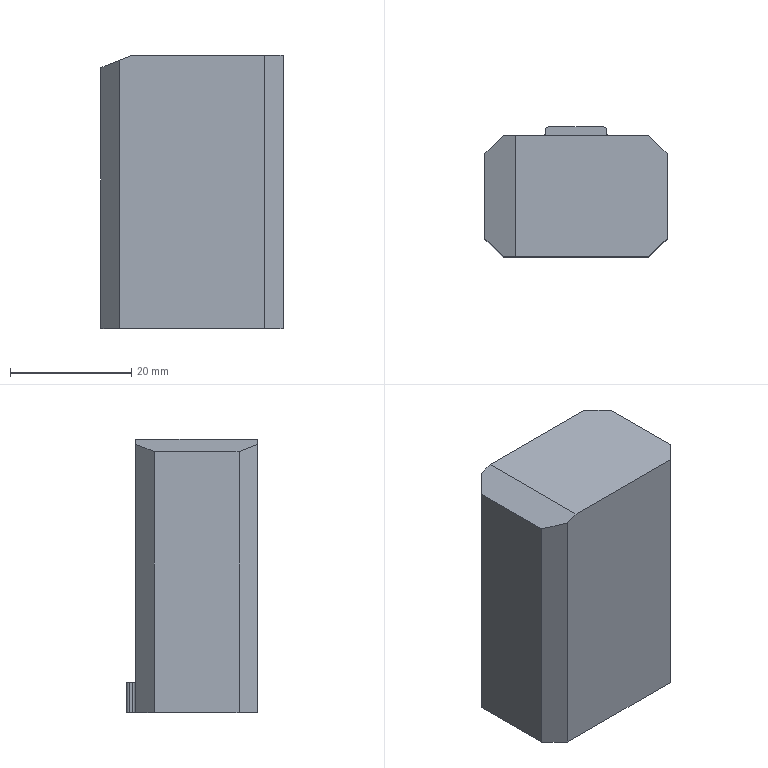Part | NX | features DIE-57 2 | 1 solid | 21 faces | box 30 x 21.5 x 45 mm | volume 25409 mm3 | plane 16 | cylinder 5 | commonest cylinder face diameters 1 x4 14.003 x1
STEP:
#1=CARTESIAN_POINT('',(3135.094,-901.123,858.716));
#2=VERTEX_POINT('',#1);
#3=CARTESIAN_POINT('',(3157.094,-901.123,858.716));
#4=VERTEX_POINT('',#3);
#5=CARTESIAN_POINT('',(3145.094,-901.123,858.716));
#6=DIRECTION('',(1.,0.,0.));
#7=VECTOR('',#6,1000.);
#8=LINE('',#5,#7);
#9=EDGE_CURVE('',#2,#4,#8,.T.);
#10=ORIENTED_EDGE('',*,*,#9,.T.);
#11=CARTESIAN_POINT('',(3160.094,-898.123,858.716));
#12=VERTEX_POINT('',#11);
#13=CARTESIAN_POINT('',(3153.594,-904.623,858.716));
#14=DIRECTION('',(0.7071,0.7071,0.));
#15=VECTOR('',#14,1000.);
#16=LINE('',#13,#15);
#17=EDGE_CURVE('',#12,#4,#16,.F.);
#18=ORIENTED_EDGE('',*,*,#17,.F.);
#19=CARTESIAN_POINT('',(3160.094,-884.123,858.716));
#20=VERTEX_POINT('',#19);
#21=CARTESIAN_POINT('',(3160.094,-891.123,858.716));
#22=DIRECTION('',(0.,1.,0.));
#23=VECTOR('',#22,1000.);
#24=LINE('',#21,#23);
#25=EDGE_CURVE('',#12,#20,#24,.T.);
#26=ORIENTED_EDGE('',*,*,#25,.T.);
#27=CARTESIAN_POINT('',(3157.094,-881.123,858.716));
#28=VERTEX_POINT('',#27);
#29=CARTESIAN_POINT('',(3153.594,-877.623,858.716));
#30=DIRECTION('',(-0.7071,0.7071,0.));
#31=VECTOR('',#30,1000.);
#32=LINE('',#29,#31);
#33=EDGE_CURVE('',#28,#20,#32,.F.);
#34=ORIENTED_EDGE('',*,*,#33,.F.);
#35=CARTESIAN_POINT('',(3135.094,-881.123,858.716));
#36=VERTEX_POINT('',#35);
#37=CARTESIAN_POINT('',(3145.094,-881.123,858.716));
#38=DIRECTION('',(-1.,0.,0.));
#39=VECTOR('',#38,1000.);
#40=LINE('',#37,#39);
#41=EDGE_CURVE('',#28,#36,#40,.T.);
#42=ORIENTED_EDGE('',*,*,#41,.T.);
#43=CARTESIAN_POINT('',(3135.094,-891.123,858.716));
#44=DIRECTION('',(0.,1.,0.));
#45=VECTOR('',#44,1000.);
#46=LINE('',#43,#45);
#47=EDGE_CURVE('',#2,#36,#46,.T.);
#48=ORIENTED_EDGE('',*,*,#47,.F.);
#49=EDGE_LOOP('',(#10,#18,#26,#34,#42,#48));
#50=FACE_BOUND('',#49,.T.);
#51=CARTESIAN_POINT('',(3145.094,-891.123,858.716));
#52=DIRECTION('',(0.,0.,1.));
#53=DIRECTION('',(1.,0.,0.));
#54=AXIS2_PLACEMENT_3D('',#51,#52,#53);
#55=PLANE('',#54);
#56=ADVANCED_FACE('',(#50),#55,.T.);
#57=CARTESIAN_POINT('',(3139.594,-881.123,818.716));
#58=VERTEX_POINT('',#57);
#59=CARTESIAN_POINT('',(3150.594,-881.123,818.716));
#60=VERTEX_POINT('',#59);
#61=CARTESIAN_POINT('',(3145.094,-881.123,818.716));
#62=DIRECTION('',(1.,0.,0.));
#63=VECTOR('',#62,1000.);
#64=LINE('',#61,#63);
#65=EDGE_CURVE('',#58,#60,#64,.T.);
#66=ORIENTED_EDGE('',*,*,#65,.F.);
#67=CARTESIAN_POINT('',(3139.594,-881.123,813.716));
#68=VERTEX_POINT('',#67);
#69=CARTESIAN_POINT('',(3139.594,-881.123,818.716));
#70=DIRECTION('',(0.,0.,-1.));
#71=VECTOR('',#70,1000.);
#72=LINE('',#69,#71);
#73=EDGE_CURVE('',#68,#58,#72,.F.);
#74=ORIENTED_EDGE('',*,*,#73,.F.);
#75=CARTESIAN_POINT('',(3133.094,-881.123,813.716));
#76=VERTEX_POINT('',#75);
#77=CARTESIAN_POINT('',(3145.094,-881.123,813.716));
#78=DIRECTION('',(1.,0.,0.));
#79=VECTOR('',#78,1000.);
#80=LINE('',#77,#79);
#81=EDGE_CURVE('',#76,#68,#80,.T.);
#82=ORIENTED_EDGE('',*,*,#81,.F.);
#83=CARTESIAN_POINT('',(3133.094,-881.123,857.916));
#84=VERTEX_POINT('',#83);
#85=CARTESIAN_POINT('',(3133.094,-881.123,823.716));
#86=DIRECTION('',(0.,0.,-1.));
#87=VECTOR('',#86,1000.);
#88=LINE('',#85,#87);
#89=EDGE_CURVE('',#84,#76,#88,.T.);
#90=ORIENTED_EDGE('',*,*,#89,.F.);
#91=CARTESIAN_POINT('',(3135.956,-881.123,859.061));
#92=DIRECTION('',(0.9285,0.,0.3714));
#93=VECTOR('',#92,1000.);
#94=LINE('',#91,#93);
#95=EDGE_CURVE('',#36,#84,#94,.F.);
#96=ORIENTED_EDGE('',*,*,#95,.F.);
#97=ORIENTED_EDGE('',*,*,#41,.F.);
#98=CARTESIAN_POINT('',(3157.094,-881.123,813.716));
#99=VERTEX_POINT('',#98);
#100=CARTESIAN_POINT('',(3157.094,-881.123,823.716));
#101=DIRECTION('',(0.,0.,1.));
#102=VECTOR('',#101,1000.);
#103=LINE('',#100,#102);
#104=EDGE_CURVE('',#99,#28,#103,.T.);
#105=ORIENTED_EDGE('',*,*,#104,.F.);
#106=CARTESIAN_POINT('',(3150.594,-881.123,813.716));
#107=VERTEX_POINT('',#106);
#108=CARTESIAN_POINT('',(3145.094,-881.123,813.716));
#109=DIRECTION('',(1.,0.,0.));
#110=VECTOR('',#109,1000.);
#111=LINE('',#108,#110);
#112=EDGE_CURVE('',#107,#99,#111,.T.);
#113=ORIENTED_EDGE('',*,*,#112,.F.);
#114=CARTESIAN_POINT('',(3150.594,-881.123,813.716));
#115=DIRECTION('',(0.,0.,1.));
#116=VECTOR('',#115,1000.);
#117=LINE('',#114,#116);
#118=EDGE_CURVE('',#60,#107,#117,.F.);
#119=ORIENTED_EDGE('',*,*,#118,.F.);
#120=EDGE_LOOP('',(#66,#74,#82,#90,#96,#97,#105,#113,#119));
#121=FACE_BOUND('',#120,.T.);
#122=CARTESIAN_POINT('',(3145.094,-881.123,823.716));
#123=DIRECTION('',(0.,1.,0.));
#124=DIRECTION('',(0.,0.,-1.));
#125=AXIS2_PLACEMENT_3D('',#122,#123,#124);
#126=PLANE('',#125);
#127=ADVANCED_FACE('',(#121),#126,.T.);
#128=CARTESIAN_POINT('',(3130.094,-884.123,813.716));
#129=VERTEX_POINT('',#128);
#130=CARTESIAN_POINT('',(3130.094,-884.123,856.716));
#131=VERTEX_POINT('',#130);
#132=CARTESIAN_POINT('',(3130.094,-884.123,823.716));
#133=DIRECTION('',(0.,0.,1.));
#134=VECTOR('',#133,1000.);
#135=LINE('',#132,#134);
#136=EDGE_CURVE('',#129,#131,#135,.T.);
#137=ORIENTED_EDGE('',*,*,#136,.F.);
#138=CARTESIAN_POINT('',(3130.094,-898.123,813.716));
#139=VERTEX_POINT('',#138);
#140=CARTESIAN_POINT('',(3130.094,-891.123,813.716));
#141=DIRECTION('',(0.,1.,0.));
#142=VECTOR('',#141,1000.);
#143=LINE('',#140,#142);
#144=EDGE_CURVE('',#139,#129,#143,.T.);
#145=ORIENTED_EDGE('',*,*,#144,.F.);
#146=CARTESIAN_POINT('',(3130.094,-898.123,856.716));
#147=VERTEX_POINT('',#146);
#148=CARTESIAN_POINT('',(3130.094,-898.123,823.716));
#149=DIRECTION('',(0.,0.,-1.));
#150=VECTOR('',#149,1000.);
#151=LINE('',#148,#150);
#152=EDGE_CURVE('',#147,#139,#151,.T.);
#153=ORIENTED_EDGE('',*,*,#152,.F.);
#154=CARTESIAN_POINT('',(3130.094,-891.123,856.716));
#155=DIRECTION('',(0.,-1.,0.));
#156=VECTOR('',#155,1000.);
#157=LINE('',#154,#156);
#158=EDGE_CURVE('',#131,#147,#157,.T.);
#159=ORIENTED_EDGE('',*,*,#158,.F.);
#160=EDGE_LOOP('',(#137,#145,#153,#159));
#161=FACE_BOUND('',#160,.T.);
#162=CARTESIAN_POINT('',(3130.094,-891.123,823.716));
#163=DIRECTION('',(-1.,0.,0.));
#164=DIRECTION('',(0.,0.,1.));
#165=AXIS2_PLACEMENT_3D('',#162,#163,#164);
#166=PLANE('',#165);
#167=ADVANCED_FACE('',(#161),#166,.T.);
#168=CARTESIAN_POINT('',(3133.094,-901.123,813.716));
#169=VERTEX_POINT('',#168);
#170=CARTESIAN_POINT('',(3133.094,-901.123,857.916));
#171=VERTEX_POINT('',#170);
#172=CARTESIAN_POINT('',(3133.094,-901.123,823.716));
#173=DIRECTION('',(0.,0.,1.));
#174=VECTOR('',#173,1000.);
#175=LINE('',#172,#174);
#176=EDGE_CURVE('',#169,#171,#175,.T.);
#177=ORIENTED_EDGE('',*,*,#176,.F.);
#178=CARTESIAN_POINT('',(3157.094,-901.123,813.716));
#179=VERTEX_POINT('',#178);
#180=CARTESIAN_POINT('',(3145.094,-901.123,813.716));
#181=DIRECTION('',(-1.,0.,0.));
#182=VECTOR('',#181,1000.);
#183=LINE('',#180,#182);
#184=EDGE_CURVE('',#179,#169,#183,.T.);
#185=ORIENTED_EDGE('',*,*,#184,.F.);
#186=CARTESIAN_POINT('',(3157.094,-901.123,823.716));
#187=DIRECTION('',(0.,0.,-1.));
#188=VECTOR('',#187,1000.);
#189=LINE('',#186,#188);
#190=EDGE_CURVE('',#4,#179,#189,.T.);
#191=ORIENTED_EDGE('',*,*,#190,.F.);
#192=ORIENTED_EDGE('',*,*,#9,.F.);
#193=CARTESIAN_POINT('',(3135.956,-901.123,859.061));
#194=DIRECTION('',(-0.9285,0.,-0.3714));
#195=VECTOR('',#194,1000.);
#196=LINE('',#193,#195);
#197=EDGE_CURVE('',#171,#2,#196,.F.);
#198=ORIENTED_EDGE('',*,*,#197,.F.);
#199=EDGE_LOOP('',(#177,#185,#191,#192,#198));
#200=FACE_BOUND('',#199,.T.);
#201=CARTESIAN_POINT('',(3145.094,-901.123,823.716));
#202=DIRECTION('',(0.,-1.,0.));
#203=DIRECTION('',(0.,0.,1.));
#204=AXIS2_PLACEMENT_3D('',#201,#202,#203);
#205=PLANE('',#204);
#206=ADVANCED_FACE('',(#200),#205,.T.);
#207=CARTESIAN_POINT('',(3138.092,-891.123,813.716));
#208=VERTEX_POINT('',#207);
#209=CARTESIAN_POINT('',(3145.094,-891.123,813.716));
#210=DIRECTION('',(0.,0.,-1.));
#211=DIRECTION('',(-1.,0.,0.));
#212=AXIS2_PLACEMENT_3D('',#209,#210,#211);
#213=CIRCLE('',#212,7.002);
#214=EDGE_CURVE('',#208,#208,#213,.F.);
#215=ORIENTED_EDGE('',*,*,#214,.T.);
#216=EDGE_LOOP('',(#215));
#217=FACE_BOUND('',#216,.T.);
#218=CARTESIAN_POINT('',(3150.094,-880.623,813.716));
#219=VERTEX_POINT('',#218);
#220=CARTESIAN_POINT('',(3150.094,-880.123,813.716));
#221=VERTEX_POINT('',#220);
#222=CARTESIAN_POINT('',(3150.094,-2118.745,813.716));
#223=DIRECTION('',(0.,1.,0.));
#224=VECTOR('',#223,1000.);
#225=LINE('',#222,#224);
#226=EDGE_CURVE('',#219,#221,#225,.T.);
#227=ORIENTED_EDGE('',*,*,#226,.F.);
#228=CARTESIAN_POINT('',(3150.594,-880.623,813.716));
#229=DIRECTION('',(0.,0.,1.));
#230=DIRECTION('',(-1.,0.,0.));
#231=AXIS2_PLACEMENT_3D('',#228,#229,#230);
#232=CIRCLE('',#231,0.5);
#233=EDGE_CURVE('',#107,#219,#232,.F.);
#234=ORIENTED_EDGE('',*,*,#233,.F.);
#235=ORIENTED_EDGE('',*,*,#112,.T.);
#236=CARTESIAN_POINT('',(3160.094,-884.123,813.716));
#237=VERTEX_POINT('',#236);
#238=CARTESIAN_POINT('',(3153.594,-877.623,813.716));
#239=DIRECTION('',(0.7071,-0.7071,0.));
#240=VECTOR('',#239,1000.);
#241=LINE('',#238,#240);
#242=EDGE_CURVE('',#237,#99,#241,.F.);
#243=ORIENTED_EDGE('',*,*,#242,.F.);
#244=CARTESIAN_POINT('',(3160.094,-898.123,813.716));
#245=VERTEX_POINT('',#244);
#246=CARTESIAN_POINT('',(3160.094,-891.123,813.716));
#247=DIRECTION('',(0.,-1.,0.));
#248=VECTOR('',#247,1000.);
#249=LINE('',#246,#248);
#250=EDGE_CURVE('',#237,#245,#249,.T.);
#251=ORIENTED_EDGE('',*,*,#250,.T.);
#252=CARTESIAN_POINT('',(3153.594,-904.623,813.716));
#253=DIRECTION('',(-0.7071,-0.7071,0.));
#254=VECTOR('',#253,1000.);
#255=LINE('',#252,#254);
#256=EDGE_CURVE('',#179,#245,#255,.F.);
#257=ORIENTED_EDGE('',*,*,#256,.F.);
#258=ORIENTED_EDGE('',*,*,#184,.T.);
#259=CARTESIAN_POINT('',(3136.594,-904.623,813.716));
#260=DIRECTION('',(-0.7071,0.7071,0.));
#261=VECTOR('',#260,1000.);
#262=LINE('',#259,#261);
#263=EDGE_CURVE('',#139,#169,#262,.F.);
#264=ORIENTED_EDGE('',*,*,#263,.F.);
#265=ORIENTED_EDGE('',*,*,#144,.T.);
#266=CARTESIAN_POINT('',(3136.594,-877.623,813.716));
#267=DIRECTION('',(0.7071,0.7071,0.));
#268=VECTOR('',#267,1000.);
#269=LINE('',#266,#268);
#270=EDGE_CURVE('',#76,#129,#269,.F.);
#271=ORIENTED_EDGE('',*,*,#270,.F.);
#272=ORIENTED_EDGE('',*,*,#81,.T.);
#273=CARTESIAN_POINT('',(3140.094,-880.623,813.716));
#274=VERTEX_POINT('',#273);
#275=CARTESIAN_POINT('',(3139.594,-880.623,813.716));
#276=DIRECTION('',(0.,0.,1.));
#277=DIRECTION('',(-1.,0.,0.));
#278=AXIS2_PLACEMENT_3D('',#275,#276,#277);
#279=CIRCLE('',#278,0.5);
#280=EDGE_CURVE('',#274,#68,#279,.F.);
#281=ORIENTED_EDGE('',*,*,#280,.F.);
#282=CARTESIAN_POINT('',(3140.094,-880.123,813.716));
#283=VERTEX_POINT('',#282);
#284=CARTESIAN_POINT('',(3140.094,-2118.745,813.716));
#285=DIRECTION('',(0.,-1.,0.));
#286=VECTOR('',#285,1000.);
#287=LINE('',#284,#286);
#288=EDGE_CURVE('',#283,#274,#287,.T.);
#289=ORIENTED_EDGE('',*,*,#288,.F.);
#290=CARTESIAN_POINT('',(3140.594,-879.623,813.716));
#291=VERTEX_POINT('',#290);
#292=CARTESIAN_POINT('',(3140.594,-880.123,813.716));
#293=DIRECTION('',(0.,0.,1.));
#294=DIRECTION('',(-1.,0.,0.));
#295=AXIS2_PLACEMENT_3D('',#292,#293,#294);
#296=CIRCLE('',#295,0.5);
#297=EDGE_CURVE('',#291,#283,#296,.T.);
#298=ORIENTED_EDGE('',*,*,#297,.F.);
#299=CARTESIAN_POINT('',(3149.594,-879.623,813.716));
#300=VERTEX_POINT('',#299);
#301=CARTESIAN_POINT('',(3145.094,-879.623,813.716));
#302=DIRECTION('',(-1.,0.,0.));
#303=VECTOR('',#302,1000.);
#304=LINE('',#301,#303);
#305=EDGE_CURVE('',#300,#291,#304,.T.);
#306=ORIENTED_EDGE('',*,*,#305,.F.);
#307=CARTESIAN_POINT('',(3149.594,-880.123,813.716));
#308=DIRECTION('',(0.,0.,1.));
#309=DIRECTION('',(-1.,0.,0.));
#310=AXIS2_PLACEMENT_3D('',#307,#308,#309);
#311=CIRCLE('',#310,0.5);
#312=EDGE_CURVE('',#221,#300,#311,.T.);
#313=ORIENTED_EDGE('',*,*,#312,.F.);
#314=EDGE_LOOP('',(#227,#234,#235,#243,#251,#257,#258,#264,#265,#271,#272,#281,#289,#298,#306,#313));
#315=FACE_BOUND('',#314,.T.);
#316=CARTESIAN_POINT('',(3145.094,-891.123,813.716));
#317=DIRECTION('',(0.,0.,-1.));
#318=DIRECTION('',(-1.,0.,0.));
#319=AXIS2_PLACEMENT_3D('',#316,#317,#318);
#320=PLANE('',#319);
#321=ADVANCED_FACE('',(#217,#315),#320,.T.);
#322=ORIENTED_EDGE('',*,*,#25,.F.);
#323=CARTESIAN_POINT('',(3160.094,-898.123,823.716));
#324=DIRECTION('',(0.,0.,1.));
#325=VECTOR('',#324,1000.);
#326=LINE('',#323,#325);
#327=EDGE_CURVE('',#245,#12,#326,.T.);
#328=ORIENTED_EDGE('',*,*,#327,.F.);
#329=ORIENTED_EDGE('',*,*,#250,.F.);
#330=CARTESIAN_POINT('',(3160.094,-884.123,823.716));
#331=DIRECTION('',(0.,0.,-1.));
#332=VECTOR('',#331,1000.);
#333=LINE('',#330,#332);
#334=EDGE_CURVE('',#20,#237,#333,.T.);
#335=ORIENTED_EDGE('',*,*,#334,.F.);
#336=EDGE_LOOP('',(#322,#328,#329,#335));
#337=FACE_BOUND('',#336,.T.);
#338=CARTESIAN_POINT('',(3160.094,-891.123,823.716));
#339=DIRECTION('',(1.,0.,0.));
#340=DIRECTION('',(0.,0.,-1.));
#341=AXIS2_PLACEMENT_3D('',#338,#339,#340);
#342=PLANE('',#341);
#343=ADVANCED_FACE('',(#337),#342,.T.);
#344=ORIENTED_EDGE('',*,*,#242,.T.);
#345=ORIENTED_EDGE('',*,*,#104,.T.);
#346=ORIENTED_EDGE('',*,*,#33,.T.);
#347=ORIENTED_EDGE('',*,*,#334,.T.);
#348=EDGE_LOOP('',(#344,#345,#346,#347));
#349=FACE_BOUND('',#348,.T.);
#350=CARTESIAN_POINT('',(3157.094,-881.123,823.716));
#351=DIRECTION('',(-0.7071,-0.7071,0.));
#352=DIRECTION('',(0.,0.,1.));
#353=AXIS2_PLACEMENT_3D('',#350,#351,#352);
#354=PLANE('',#353);
#355=ADVANCED_FACE('',(#349),#354,.F.);
#356=ORIENTED_EDGE('',*,*,#256,.T.);
#357=ORIENTED_EDGE('',*,*,#327,.T.);
#358=ORIENTED_EDGE('',*,*,#17,.T.);
#359=ORIENTED_EDGE('',*,*,#190,.T.);
#360=EDGE_LOOP('',(#356,#357,#358,#359));
#361=FACE_BOUND('',#360,.T.);
#362=CARTESIAN_POINT('',(3160.094,-898.123,823.716));
#363=DIRECTION('',(-0.7071,0.7071,0.));
#364=DIRECTION('',(0.,0.,1.));
#365=AXIS2_PLACEMENT_3D('',#362,#363,#364);
#366=PLANE('',#365);
#367=ADVANCED_FACE('',(#361),#366,.F.);
#368=ORIENTED_EDGE('',*,*,#152,.T.);
#369=ORIENTED_EDGE('',*,*,#263,.T.);
#370=ORIENTED_EDGE('',*,*,#176,.T.);
#371=CARTESIAN_POINT('',(3126.761,-894.789,855.383));
#372=DIRECTION('',(0.6804,-0.6804,0.2722));
#373=VECTOR('',#372,1000.);
#374=LINE('',#371,#373);
#375=EDGE_CURVE('',#147,#171,#374,.T.);
#376=ORIENTED_EDGE('',*,*,#375,.F.);
#377=EDGE_LOOP('',(#368,#369,#370,#376));
#378=FACE_BOUND('',#377,.T.);
#379=CARTESIAN_POINT('',(3133.094,-901.123,823.716));
#380=DIRECTION('',(0.7071,0.7071,0.));
#381=DIRECTION('',(0.,0.,1.));
#382=AXIS2_PLACEMENT_3D('',#379,#380,#381);
#383=PLANE('',#382);
#384=ADVANCED_FACE('',(#378),#383,.F.);
#385=ORIENTED_EDGE('',*,*,#89,.T.);
#386=ORIENTED_EDGE('',*,*,#270,.T.);
#387=ORIENTED_EDGE('',*,*,#136,.T.);
#388=CARTESIAN_POINT('',(3123.983,-890.234,854.272));
#389=DIRECTION('',(-0.6804,-0.6804,-0.2722));
#390=VECTOR('',#389,1000.);
#391=LINE('',#388,#390);
#392=EDGE_CURVE('',#84,#131,#391,.T.);
#393=ORIENTED_EDGE('',*,*,#392,.F.);
#394=EDGE_LOOP('',(#385,#386,#387,#393));
#395=FACE_BOUND('',#394,.T.);
#396=CARTESIAN_POINT('',(3130.094,-884.123,823.716));
#397=DIRECTION('',(0.7071,-0.7071,0.));
#398=DIRECTION('',(0.,0.,1.));
#399=AXIS2_PLACEMENT_3D('',#396,#397,#398);
#400=PLANE('',#399);
#401=ADVANCED_FACE('',(#395),#400,.F.);
#402=ORIENTED_EDGE('',*,*,#95,.T.);
#403=ORIENTED_EDGE('',*,*,#392,.T.);
#404=ORIENTED_EDGE('',*,*,#158,.T.);
#405=ORIENTED_EDGE('',*,*,#375,.T.);
#406=ORIENTED_EDGE('',*,*,#197,.T.);
#407=ORIENTED_EDGE('',*,*,#47,.T.);
#408=EDGE_LOOP('',(#402,#403,#404,#405,#406,#407));
#409=FACE_BOUND('',#408,.T.);
#410=CARTESIAN_POINT('',(3130.094,-891.123,856.716));
#411=DIRECTION('',(0.3714,0.,-0.9285));
#412=DIRECTION('',(0.,-1.,0.));
#413=AXIS2_PLACEMENT_3D('',#410,#411,#412);
#414=PLANE('',#413);
#415=ADVANCED_FACE('',(#409),#414,.F.);
#416=CARTESIAN_POINT('',(3140.094,-880.123,818.716));
#417=VERTEX_POINT('',#416);
#418=CARTESIAN_POINT('',(3140.094,-880.623,818.716));
#419=VERTEX_POINT('',#418);
#420=CARTESIAN_POINT('',(3140.094,-2118.745,818.716));
#421=DIRECTION('',(0.,-1.,0.));
#422=VECTOR('',#421,1000.);
#423=LINE('',#420,#422);
#424=EDGE_CURVE('',#417,#419,#423,.T.);
#425=ORIENTED_EDGE('',*,*,#424,.F.);
#426=CARTESIAN_POINT('',(3140.094,-880.123,818.716));
#427=DIRECTION('',(0.,0.,-1.));
#428=VECTOR('',#427,1000.);
#429=LINE('',#426,#428);
#430=EDGE_CURVE('',#283,#417,#429,.F.);
#431=ORIENTED_EDGE('',*,*,#430,.F.);
#432=ORIENTED_EDGE('',*,*,#288,.T.);
#433=CARTESIAN_POINT('',(3140.094,-880.623,813.716));
#434=DIRECTION('',(0.,0.,-1.));
#435=VECTOR('',#434,1000.);
#436=LINE('',#433,#435);
#437=EDGE_CURVE('',#419,#274,#436,.T.);
#438=ORIENTED_EDGE('',*,*,#437,.F.);
#439=EDGE_LOOP('',(#425,#431,#432,#438));
#440=FACE_BOUND('',#439,.T.);
#441=CARTESIAN_POINT('',(3140.094,-880.123,818.716));
#442=DIRECTION('',(-1.,0.,0.));
#443=DIRECTION('',(0.,0.,1.));
#444=AXIS2_PLACEMENT_3D('',#441,#442,#443);
#445=PLANE('',#444);
#446=ADVANCED_FACE('',(#440),#445,.T.);
#447=CARTESIAN_POINT('',(3150.094,-880.623,818.716));
#448=VERTEX_POINT('',#447);
#449=CARTESIAN_POINT('',(3150.094,-880.123,818.716));
#450=VERTEX_POINT('',#449);
#451=CARTESIAN_POINT('',(3150.094,-2118.745,818.716));
#452=DIRECTION('',(0.,1.,0.));
#453=VECTOR('',#452,1000.);
#454=LINE('',#451,#453);
#455=EDGE_CURVE('',#448,#450,#454,.T.);
#456=ORIENTED_EDGE('',*,*,#455,.F.);
#457=CARTESIAN_POINT('',(3150.094,-880.623,818.716));
#458=DIRECTION('',(0.,0.,1.));
#459=VECTOR('',#458,1000.);
#460=LINE('',#457,#459);
#461=EDGE_CURVE('',#219,#448,#460,.T.);
#462=ORIENTED_EDGE('',*,*,#461,.F.);
#463=ORIENTED_EDGE('',*,*,#226,.T.);
#464=CARTESIAN_POINT('',(3150.094,-880.123,818.716));
#465=DIRECTION('',(0.,0.,-1.));
#466=VECTOR('',#465,1000.);
#467=LINE('',#464,#466);
#468=EDGE_CURVE('',#450,#221,#467,.T.);
#469=ORIENTED_EDGE('',*,*,#468,.F.);
#470=EDGE_LOOP('',(#456,#462,#463,#469));
#471=FACE_BOUND('',#470,.T.);
#472=CARTESIAN_POINT('',(3150.094,-881.173,818.716));
#473=DIRECTION('',(1.,0.,0.));
#474=DIRECTION('',(0.,0.,-1.));
#475=AXIS2_PLACEMENT_3D('',#472,#473,#474);
#476=PLANE('',#475);
#477=ADVANCED_FACE('',(#471),#476,.T.);
#478=ORIENTED_EDGE('',*,*,#305,.T.);
#479=CARTESIAN_POINT('',(3140.594,-879.623,818.716));
#480=VERTEX_POINT('',#479);
#481=CARTESIAN_POINT('',(3140.594,-879.623,818.716));
#482=DIRECTION('',(0.,0.,-1.));
#483=VECTOR('',#482,1000.);
#484=LINE('',#481,#483);
#485=EDGE_CURVE('',#480,#291,#484,.T.);
#486=ORIENTED_EDGE('',*,*,#485,.F.);
#487=CARTESIAN_POINT('',(3149.594,-879.623,818.716));
#488=VERTEX_POINT('',#487);
#489=CARTESIAN_POINT('',(962.5,-879.623,818.716));
#490=DIRECTION('',(-1.,0.,0.));
#491=VECTOR('',#490,1000.);
#492=LINE('',#489,#491);
#493=EDGE_CURVE('',#488,#480,#492,.T.);
#494=ORIENTED_EDGE('',*,*,#493,.F.);
#495=CARTESIAN_POINT('',(3149.594,-879.623,818.716));
#496=DIRECTION('',(0.,0.,-1.));
#497=VECTOR('',#496,1000.);
#498=LINE('',#495,#497);
#499=EDGE_CURVE('',#300,#488,#498,.F.);
#500=ORIENTED_EDGE('',*,*,#499,.F.);
#501=EDGE_LOOP('',(#478,#486,#494,#500));
#502=FACE_BOUND('',#501,.T.);
#503=CARTESIAN_POINT('',(3162.094,-879.623,818.716));
#504=DIRECTION('',(0.,1.,0.));
#505=DIRECTION('',(0.,0.,-1.));
#506=AXIS2_PLACEMENT_3D('',#503,#504,#505);
#507=PLANE('',#506);
#508=ADVANCED_FACE('',(#502),#507,.T.);
#509=ORIENTED_EDGE('',*,*,#493,.T.);
#510=CARTESIAN_POINT('',(3140.594,-880.123,818.716));
#511=DIRECTION('',(0.,0.,1.));
#512=DIRECTION('',(-1.,0.,0.));
#513=AXIS2_PLACEMENT_3D('',#510,#511,#512);
#514=CIRCLE('',#513,0.5);
#515=EDGE_CURVE('',#417,#480,#514,.F.);
#516=ORIENTED_EDGE('',*,*,#515,.F.);
#517=ORIENTED_EDGE('',*,*,#424,.T.);
#518=CARTESIAN_POINT('',(3139.594,-880.623,818.716));
#519=DIRECTION('',(0.,0.,1.));
#520=DIRECTION('',(-1.,0.,0.));
#521=AXIS2_PLACEMENT_3D('',#518,#519,#520);
#522=CIRCLE('',#521,0.5);
#523=EDGE_CURVE('',#58,#419,#522,.T.);
#524=ORIENTED_EDGE('',*,*,#523,.F.);
#525=ORIENTED_EDGE('',*,*,#65,.T.);
#526=CARTESIAN_POINT('',(3150.594,-880.623,818.716));
#527=DIRECTION('',(0.,0.,1.));
#528=DIRECTION('',(-1.,0.,0.));
#529=AXIS2_PLACEMENT_3D('',#526,#527,#528);
#530=CIRCLE('',#529,0.5);
#531=EDGE_CURVE('',#448,#60,#530,.T.);
#532=ORIENTED_EDGE('',*,*,#531,.F.);
#533=ORIENTED_EDGE('',*,*,#455,.T.);
#534=CARTESIAN_POINT('',(3149.594,-880.123,818.716));
#535=DIRECTION('',(0.,0.,1.));
#536=DIRECTION('',(-1.,0.,0.));
#537=AXIS2_PLACEMENT_3D('',#534,#535,#536);
#538=CIRCLE('',#537,0.5);
#539=EDGE_CURVE('',#488,#450,#538,.F.);
#540=ORIENTED_EDGE('',*,*,#539,.F.);
#541=EDGE_LOOP('',(#509,#516,#517,#524,#525,#532,#533,#540));
#542=FACE_BOUND('',#541,.T.);
#543=CARTESIAN_POINT('',(962.5,-2118.745,818.716));
#544=DIRECTION('',(0.,0.,-1.));
#545=DIRECTION('',(-1.,0.,0.));
#546=AXIS2_PLACEMENT_3D('',#543,#544,#545);
#547=PLANE('',#546);
#548=ADVANCED_FACE('',(#542),#547,.F.);
#549=ORIENTED_EDGE('',*,*,#539,.T.);
#550=ORIENTED_EDGE('',*,*,#468,.T.);
#551=ORIENTED_EDGE('',*,*,#312,.T.);
#552=ORIENTED_EDGE('',*,*,#499,.T.);
#553=EDGE_LOOP('',(#549,#550,#551,#552));
#554=FACE_BOUND('',#553,.T.);
#555=CARTESIAN_POINT('',(3149.594,-880.123,818.716));
#556=DIRECTION('',(0.,0.,-1.));
#557=DIRECTION('',(-1.,0.,0.));
#558=AXIS2_PLACEMENT_3D('',#555,#556,#557);
#559=CYLINDRICAL_SURFACE('',#558,0.5);
#560=ADVANCED_FACE('',(#554),#559,.T.);
#561=ORIENTED_EDGE('',*,*,#233,.T.);
#562=ORIENTED_EDGE('',*,*,#461,.T.);
#563=ORIENTED_EDGE('',*,*,#531,.T.);
#564=ORIENTED_EDGE('',*,*,#118,.T.);
#565=EDGE_LOOP('',(#561,#562,#563,#564));
#566=FACE_BOUND('',#565,.T.);
#567=CARTESIAN_POINT('',(3150.594,-880.623,818.716));
#568=DIRECTION('',(0.,0.,-1.));
#569=DIRECTION('',(-1.,0.,0.));
#570=AXIS2_PLACEMENT_3D('',#567,#568,#569);
#571=CYLINDRICAL_SURFACE('',#570,0.5);
#572=ADVANCED_FACE('',(#566),#571,.F.);
#573=ORIENTED_EDGE('',*,*,#523,.T.);
#574=ORIENTED_EDGE('',*,*,#437,.T.);
#575=ORIENTED_EDGE('',*,*,#280,.T.);
#576=ORIENTED_EDGE('',*,*,#73,.T.);
#577=EDGE_LOOP('',(#573,#574,#575,#576));
#578=FACE_BOUND('',#577,.T.);
#579=CARTESIAN_POINT('',(3139.594,-880.623,818.716));
#580=DIRECTION('',(0.,0.,1.));
#581=DIRECTION('',(1.,0.,0.));
#582=AXIS2_PLACEMENT_3D('',#579,#580,#581);
#583=CYLINDRICAL_SURFACE('',#582,0.5);
#584=ADVANCED_FACE('',(#578),#583,.F.);
#585=ORIENTED_EDGE('',*,*,#515,.T.);
#586=ORIENTED_EDGE('',*,*,#485,.T.);
#587=ORIENTED_EDGE('',*,*,#297,.T.);
#588=ORIENTED_EDGE('',*,*,#430,.T.);
#589=EDGE_LOOP('',(#585,#586,#587,#588));
#590=FACE_BOUND('',#589,.T.);
#591=CARTESIAN_POINT('',(3140.594,-880.123,818.716));
#592=DIRECTION('',(0.,0.,-1.));
#593=DIRECTION('',(-1.,0.,0.));
#594=AXIS2_PLACEMENT_3D('',#591,#592,#593);
#595=CYLINDRICAL_SURFACE('',#594,0.5);
#596=ADVANCED_FACE('',(#590),#595,.T.);
#597=CARTESIAN_POINT('',(3152.095,-891.123,818.716));
#598=VERTEX_POINT('',#597);
#599=CARTESIAN_POINT('',(3145.094,-891.123,818.716));
#600=DIRECTION('',(0.,0.,-1.));
#601=DIRECTION('',(1.,0.,0.));
#602=AXIS2_PLACEMENT_3D('',#599,#600,#601);
#603=CIRCLE('',#602,7.002);
#604=EDGE_CURVE('',#598,#598,#603,.F.);
#605=ORIENTED_EDGE('',*,*,#604,.F.);
#606=EDGE_LOOP('',(#605));
#607=FACE_BOUND('',#606,.T.);
#608=CARTESIAN_POINT('',(3145.094,-891.123,818.716));
#609=DIRECTION('',(0.,0.,1.));
#610=DIRECTION('',(1.,0.,0.));
#611=AXIS2_PLACEMENT_3D('',#608,#609,#610);
#612=PLANE('',#611);
#613=ADVANCED_FACE('',(#607),#612,.F.);
#614=ORIENTED_EDGE('',*,*,#604,.T.);
#615=EDGE_LOOP('',(#614));
#616=FACE_BOUND('',#615,.T.);
#617=ORIENTED_EDGE('',*,*,#214,.F.);
#618=EDGE_LOOP('',(#617));
#619=FACE_BOUND('',#618,.T.);
#620=CARTESIAN_POINT('',(3145.094,-891.123,818.716));
#621=DIRECTION('',(0.,0.,-1.));
#622=DIRECTION('',(1.,0.,0.));
#623=AXIS2_PLACEMENT_3D('',#620,#621,#622);
#624=CYLINDRICAL_SURFACE('',#623,7.002);
#625=ADVANCED_FACE('',(#616,#619),#624,.F.);
#626=CLOSED_SHELL('',(#56,#127,#167,#206,#321,#343,#355,#367,#384,#401,#415,#446,#477,#508,#548,#560,#572,#584,#596,#613,#625));
#627=MANIFOLD_SOLID_BREP('',#626);
#628=(LENGTH_UNIT()NAMED_UNIT(*)SI_UNIT(.MILLI.,.METRE.));
#629=UNCERTAINTY_MEASURE_WITH_UNIT(LENGTH_MEASURE(0.00001),#628,'','');
#630=(NAMED_UNIT(*)PLANE_ANGLE_UNIT()SI_UNIT($,.RADIAN.));
#631=(NAMED_UNIT(*)SI_UNIT($,.STERADIAN.)SOLID_ANGLE_UNIT());
#632=(GEOMETRIC_REPRESENTATION_CONTEXT(3)GLOBAL_UNCERTAINTY_ASSIGNED_CONTEXT((#629))GLOBAL_UNIT_ASSIGNED_CONTEXT((#628,#630,#631))REPRESENTATION_CONTEXT('',''));
#633=ADVANCED_BREP_SHAPE_REPRESENTATION('',(#627),#632);